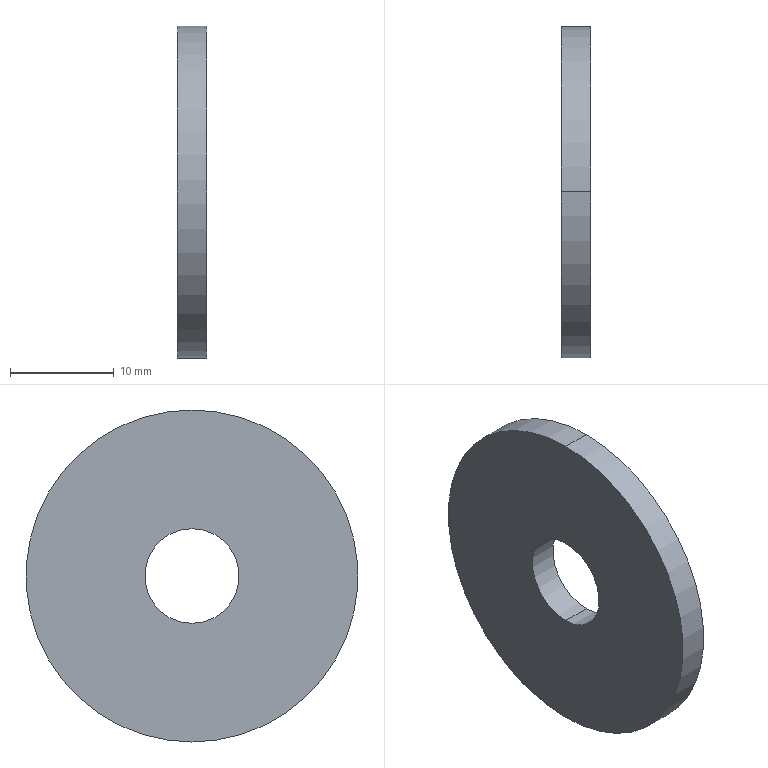Part | STEP file | flat washer wide_am_B18.22M - Plain washer, 8 mm, wide | 1 solid | 6 faces | box 2.8 x 32 x 32 mm | volume 2069 mm3 | cylinder 4 | plane 2 | commonest cylinder face diameters 9.12 x2 32 x2
STEP:
#1=CARTESIAN_POINT('',(0.,0.,0.));
#2=DIRECTION('',(0.,0.,1.));
#3=DIRECTION('',(1.,0.,0.));
#4=AXIS2_PLACEMENT_3D('',#1,#2,#3);
#5=CARTESIAN_POINT('',(0.,0.,16.));
#6=VERTEX_POINT('',#5);
#7=CARTESIAN_POINT('',(0.,0.,-16.));
#8=VERTEX_POINT('',#7);
#9=CARTESIAN_POINT('',(0.,0.,0.));
#10=DIRECTION('',(-1.,0.,0.));
#11=DIRECTION('',(0.,0.,1.));
#12=AXIS2_PLACEMENT_3D('',#9,#10,#11);
#13=CIRCLE('',#12,16.);
#14=CARTESIAN_POINT('',(-34.925,0.,0.));
#15=DIRECTION('',(-1.,0.,0.));
#16=DIRECTION('',(0.,0.,1.));
#17=AXIS2_PLACEMENT_3D('',#14,#15,#16);
#18=CYLINDRICAL_SURFACE('',#17,16.);
#19=CARTESIAN_POINT('',(0.,-34.925));
#20=DIRECTION('',(1.,0.));
#21=VECTOR('',#20,1.);
#22=LINE('',#19,#21);
#23=(GEOMETRIC_REPRESENTATION_CONTEXT(2)PARAMETRIC_REPRESENTATION_CONTEXT()REPRESENTATION_CONTEXT('',''));
#24=DEFINITIONAL_REPRESENTATION('',(#22),#23);
#25=PCURVE('',#18,#24);
#26=CARTESIAN_POINT('',(0.,4.56,0.));
#27=DIRECTION('',(-1.,0.,0.));
#28=DIRECTION('',(0.,0.,1.));
#29=AXIS2_PLACEMENT_3D('',#26,#27,#28);
#30=PLANE('',#29);
#31=CARTESIAN_POINT('',(0.,-4.56));
#32=DIRECTION('',(1.,0.));
#33=AXIS2_PLACEMENT_2D('',#31,#32);
#34=CIRCLE('',#33,16.);
#35=(GEOMETRIC_REPRESENTATION_CONTEXT(2)PARAMETRIC_REPRESENTATION_CONTEXT()REPRESENTATION_CONTEXT('',''));
#36=DEFINITIONAL_REPRESENTATION('',(#34),#35);
#37=PCURVE('',#30,#36);
#38=SURFACE_CURVE('',#13,(#25,#37),.PCURVE_S1.);
#39=EDGE_CURVE('',#6,#8,#38,.T.);
#40=ORIENTED_EDGE('',*,*,#39,.T.);
#41=CARTESIAN_POINT('',(-2.8,0.,-16.));
#42=VERTEX_POINT('',#41);
#43=CARTESIAN_POINT('',(-34.925,0.,-16.));
#44=DIRECTION('',(-1.,0.,0.));
#45=VECTOR('',#44,1.);
#46=LINE('',#43,#45);
#47=CARTESIAN_POINT('',(3.142,0.));
#48=DIRECTION('',(0.,1.));
#49=VECTOR('',#48,1.);
#50=LINE('',#47,#49);
#51=(GEOMETRIC_REPRESENTATION_CONTEXT(2)PARAMETRIC_REPRESENTATION_CONTEXT()REPRESENTATION_CONTEXT('',''));
#52=DEFINITIONAL_REPRESENTATION('',(#50),#51);
#53=PCURVE('',#18,#52);
#54=CARTESIAN_POINT('',(-34.925,0.,0.));
#55=DIRECTION('',(-1.,0.,0.));
#56=DIRECTION('',(0.,0.,1.));
#57=AXIS2_PLACEMENT_3D('',#54,#55,#56);
#58=CYLINDRICAL_SURFACE('',#57,16.);
#59=CARTESIAN_POINT('',(3.142,0.));
#60=DIRECTION('',(0.,1.));
#61=VECTOR('',#60,1.);
#62=LINE('',#59,#61);
#63=(GEOMETRIC_REPRESENTATION_CONTEXT(2)PARAMETRIC_REPRESENTATION_CONTEXT()REPRESENTATION_CONTEXT('',''));
#64=DEFINITIONAL_REPRESENTATION('',(#62),#63);
#65=PCURVE('',#58,#64);
#66=SURFACE_CURVE('',#46,(#53,#65),.PCURVE_S1.);
#67=EDGE_CURVE('',#8,#42,#66,.T.);
#68=ORIENTED_EDGE('',*,*,#67,.T.);
#69=CARTESIAN_POINT('',(-2.8,0.,16.));
#70=VERTEX_POINT('',#69);
#71=CARTESIAN_POINT('',(-2.8,0.,0.));
#72=DIRECTION('',(-1.,0.,0.));
#73=DIRECTION('',(0.,0.,1.));
#74=AXIS2_PLACEMENT_3D('',#71,#72,#73);
#75=CIRCLE('',#74,16.);
#76=CARTESIAN_POINT('',(0.,-32.125));
#77=DIRECTION('',(1.,0.));
#78=VECTOR('',#77,1.);
#79=LINE('',#76,#78);
#80=(GEOMETRIC_REPRESENTATION_CONTEXT(2)PARAMETRIC_REPRESENTATION_CONTEXT()REPRESENTATION_CONTEXT('',''));
#81=DEFINITIONAL_REPRESENTATION('',(#79),#80);
#82=PCURVE('',#18,#81);
#83=CARTESIAN_POINT('',(-2.8,16.,0.));
#84=DIRECTION('',(1.,0.,0.));
#85=DIRECTION('',(0.,0.,-1.));
#86=AXIS2_PLACEMENT_3D('',#83,#84,#85);
#87=PLANE('',#86);
#88=CARTESIAN_POINT('',(-16.,-16.));
#89=CARTESIAN_POINT('',(-16.,11.713));
#90=CARTESIAN_POINT('',(8.,-2.144));
#91=CARTESIAN_POINT('',(32.,-16.));
#92=CARTESIAN_POINT('',(8.,-29.856));
#93=CARTESIAN_POINT('',(-16.,-43.713));
#94=CARTESIAN_POINT('',(-16.,-16.));
#95=(BOUNDED_CURVE()B_SPLINE_CURVE(2,(#88,#89,#90,#91,#92,#93,#94),.UNSPECIFIED.,.T.,.F.)B_SPLINE_CURVE_WITH_KNOTS((1,2,2,2,2,1),(-2.094,0.,2.094,4.189,6.283,8.378),.UNSPECIFIED.)CURVE()GEOMETRIC_REPRESENTATION_ITEM()RATIONAL_B_SPLINE_CURVE((1.,0.5,1.,0.5,1.,0.5,1.))REPRESENTATION_ITEM(''));
#96=(GEOMETRIC_REPRESENTATION_CONTEXT(2)PARAMETRIC_REPRESENTATION_CONTEXT()REPRESENTATION_CONTEXT('',''));
#97=DEFINITIONAL_REPRESENTATION('',(#95),#96);
#98=PCURVE('',#87,#97);
#99=SURFACE_CURVE('',#75,(#82,#98),.PCURVE_S1.);
#100=EDGE_CURVE('',#70,#42,#99,.T.);
#101=ORIENTED_EDGE('',*,*,#100,.F.);
#102=CARTESIAN_POINT('',(-34.925,0.,16.));
#103=DIRECTION('',(-1.,0.,0.));
#104=VECTOR('',#103,1.);
#105=LINE('',#102,#104);
#106=CARTESIAN_POINT('',(0.,0.));
#107=DIRECTION('',(0.,1.));
#108=VECTOR('',#107,1.);
#109=LINE('',#106,#108);
#110=(GEOMETRIC_REPRESENTATION_CONTEXT(2)PARAMETRIC_REPRESENTATION_CONTEXT()REPRESENTATION_CONTEXT('',''));
#111=DEFINITIONAL_REPRESENTATION('',(#109),#110);
#112=PCURVE('',#18,#111);
#113=CARTESIAN_POINT('',(6.283,0.));
#114=DIRECTION('',(0.,1.));
#115=VECTOR('',#114,1.);
#116=LINE('',#113,#115);
#117=(GEOMETRIC_REPRESENTATION_CONTEXT(2)PARAMETRIC_REPRESENTATION_CONTEXT()REPRESENTATION_CONTEXT('',''));
#118=DEFINITIONAL_REPRESENTATION('',(#116),#117);
#119=PCURVE('',#58,#118);
#120=SURFACE_CURVE('',#105,(#112,#119),.PCURVE_S1.);
#121=EDGE_CURVE('',#6,#70,#120,.T.);
#122=ORIENTED_EDGE('',*,*,#121,.F.);
#123=EDGE_LOOP('',(#40,#68,#101,#122));
#124=FACE_BOUND('',#123,.T.);
#125=ADVANCED_FACE('',(#124),#18,.T.);
#126=CARTESIAN_POINT('',(0.,0.,4.56));
#127=VERTEX_POINT('',#126);
#128=CARTESIAN_POINT('',(-2.8,0.,4.56));
#129=VERTEX_POINT('',#128);
#130=CARTESIAN_POINT('',(-34.925,0.,4.56));
#131=DIRECTION('',(-1.,0.,0.));
#132=VECTOR('',#131,1.);
#133=LINE('',#130,#132);
#134=CARTESIAN_POINT('',(-34.925,0.,0.));
#135=DIRECTION('',(-1.,0.,0.));
#136=DIRECTION('',(0.,0.,1.));
#137=AXIS2_PLACEMENT_3D('',#134,#135,#136);
#138=CYLINDRICAL_SURFACE('',#137,4.56);
#139=CARTESIAN_POINT('',(6.283,0.));
#140=DIRECTION('',(0.,1.));
#141=VECTOR('',#140,1.);
#142=LINE('',#139,#141);
#143=(GEOMETRIC_REPRESENTATION_CONTEXT(2)PARAMETRIC_REPRESENTATION_CONTEXT()REPRESENTATION_CONTEXT('',''));
#144=DEFINITIONAL_REPRESENTATION('',(#142),#143);
#145=PCURVE('',#138,#144);
#146=CARTESIAN_POINT('',(-34.925,0.,0.));
#147=DIRECTION('',(-1.,0.,0.));
#148=DIRECTION('',(0.,0.,1.));
#149=AXIS2_PLACEMENT_3D('',#146,#147,#148);
#150=CYLINDRICAL_SURFACE('',#149,4.56);
#151=CARTESIAN_POINT('',(0.,0.));
#152=DIRECTION('',(0.,1.));
#153=VECTOR('',#152,1.);
#154=LINE('',#151,#153);
#155=(GEOMETRIC_REPRESENTATION_CONTEXT(2)PARAMETRIC_REPRESENTATION_CONTEXT()REPRESENTATION_CONTEXT('',''));
#156=DEFINITIONAL_REPRESENTATION('',(#154),#155);
#157=PCURVE('',#150,#156);
#158=SURFACE_CURVE('',#133,(#145,#157),.PCURVE_S1.);
#159=EDGE_CURVE('',#127,#129,#158,.T.);
#160=ORIENTED_EDGE('',*,*,#159,.T.);
#161=CARTESIAN_POINT('',(-2.8,0.,-4.56));
#162=VERTEX_POINT('',#161);
#163=CARTESIAN_POINT('',(-2.8,0.,0.));
#164=DIRECTION('',(-1.,0.,0.));
#165=DIRECTION('',(0.,0.,1.));
#166=AXIS2_PLACEMENT_3D('',#163,#164,#165);
#167=CIRCLE('',#166,4.56);
#168=CARTESIAN_POINT('',(0.,-32.125));
#169=DIRECTION('',(1.,0.));
#170=VECTOR('',#169,1.);
#171=LINE('',#168,#170);
#172=(GEOMETRIC_REPRESENTATION_CONTEXT(2)PARAMETRIC_REPRESENTATION_CONTEXT()REPRESENTATION_CONTEXT('',''));
#173=DEFINITIONAL_REPRESENTATION('',(#171),#172);
#174=PCURVE('',#138,#173);
#175=CARTESIAN_POINT('',(-4.56,-16.));
#176=CARTESIAN_POINT('',(-4.56,-8.102));
#177=CARTESIAN_POINT('',(2.28,-12.051));
#178=CARTESIAN_POINT('',(9.12,-16.));
#179=CARTESIAN_POINT('',(2.28,-19.949));
#180=CARTESIAN_POINT('',(-4.56,-23.898));
#181=CARTESIAN_POINT('',(-4.56,-16.));
#182=(BOUNDED_CURVE()B_SPLINE_CURVE(2,(#175,#176,#177,#178,#179,#180,#181),.UNSPECIFIED.,.T.,.F.)B_SPLINE_CURVE_WITH_KNOTS((1,2,2,2,2,1),(-2.094,0.,2.094,4.189,6.283,8.378),.UNSPECIFIED.)CURVE()GEOMETRIC_REPRESENTATION_ITEM()RATIONAL_B_SPLINE_CURVE((1.,0.5,1.,0.5,1.,0.5,1.))REPRESENTATION_ITEM(''));
#183=(GEOMETRIC_REPRESENTATION_CONTEXT(2)PARAMETRIC_REPRESENTATION_CONTEXT()REPRESENTATION_CONTEXT('',''));
#184=DEFINITIONAL_REPRESENTATION('',(#182),#183);
#185=PCURVE('',#87,#184);
#186=SURFACE_CURVE('',#167,(#174,#185),.PCURVE_S1.);
#187=EDGE_CURVE('',#162,#129,#186,.T.);
#188=ORIENTED_EDGE('',*,*,#187,.F.);
#189=CARTESIAN_POINT('',(0.,0.,-4.56));
#190=VERTEX_POINT('',#189);
#191=CARTESIAN_POINT('',(-34.925,0.,-4.56));
#192=DIRECTION('',(-1.,0.,0.));
#193=VECTOR('',#192,1.);
#194=LINE('',#191,#193);
#195=CARTESIAN_POINT('',(3.142,0.));
#196=DIRECTION('',(0.,1.));
#197=VECTOR('',#196,1.);
#198=LINE('',#195,#197);
#199=(GEOMETRIC_REPRESENTATION_CONTEXT(2)PARAMETRIC_REPRESENTATION_CONTEXT()REPRESENTATION_CONTEXT('',''));
#200=DEFINITIONAL_REPRESENTATION('',(#198),#199);
#201=PCURVE('',#138,#200);
#202=CARTESIAN_POINT('',(3.142,0.));
#203=DIRECTION('',(0.,1.));
#204=VECTOR('',#203,1.);
#205=LINE('',#202,#204);
#206=(GEOMETRIC_REPRESENTATION_CONTEXT(2)PARAMETRIC_REPRESENTATION_CONTEXT()REPRESENTATION_CONTEXT('',''));
#207=DEFINITIONAL_REPRESENTATION('',(#205),#206);
#208=PCURVE('',#150,#207);
#209=SURFACE_CURVE('',#194,(#201,#208),.PCURVE_S1.);
#210=EDGE_CURVE('',#190,#162,#209,.T.);
#211=ORIENTED_EDGE('',*,*,#210,.F.);
#212=CARTESIAN_POINT('',(0.,0.,0.));
#213=DIRECTION('',(-1.,0.,0.));
#214=DIRECTION('',(0.,0.,1.));
#215=AXIS2_PLACEMENT_3D('',#212,#213,#214);
#216=CIRCLE('',#215,4.56);
#217=CARTESIAN_POINT('',(0.,-34.925));
#218=DIRECTION('',(1.,0.));
#219=VECTOR('',#218,1.);
#220=LINE('',#217,#219);
#221=(GEOMETRIC_REPRESENTATION_CONTEXT(2)PARAMETRIC_REPRESENTATION_CONTEXT()REPRESENTATION_CONTEXT('',''));
#222=DEFINITIONAL_REPRESENTATION('',(#220),#221);
#223=PCURVE('',#138,#222);
#224=CARTESIAN_POINT('',(0.,-4.56));
#225=DIRECTION('',(1.,0.));
#226=AXIS2_PLACEMENT_2D('',#224,#225);
#227=CIRCLE('',#226,4.56);
#228=(GEOMETRIC_REPRESENTATION_CONTEXT(2)PARAMETRIC_REPRESENTATION_CONTEXT()REPRESENTATION_CONTEXT('',''));
#229=DEFINITIONAL_REPRESENTATION('',(#227),#228);
#230=PCURVE('',#30,#229);
#231=SURFACE_CURVE('',#216,(#223,#230),.PCURVE_S1.);
#232=EDGE_CURVE('',#190,#127,#231,.T.);
#233=ORIENTED_EDGE('',*,*,#232,.T.);
#234=EDGE_LOOP('',(#160,#188,#211,#233));
#235=FACE_BOUND('',#234,.F.);
#236=ADVANCED_FACE('',(#235),#138,.F.);
#237=CARTESIAN_POINT('',(-2.8,0.,0.));
#238=DIRECTION('',(-1.,0.,0.));
#239=DIRECTION('',(0.,0.,1.));
#240=AXIS2_PLACEMENT_3D('',#237,#238,#239);
#241=CIRCLE('',#240,4.56);
#242=CARTESIAN_POINT('',(0.,-32.125));
#243=DIRECTION('',(1.,0.));
#244=VECTOR('',#243,1.);
#245=LINE('',#242,#244);
#246=(GEOMETRIC_REPRESENTATION_CONTEXT(2)PARAMETRIC_REPRESENTATION_CONTEXT()REPRESENTATION_CONTEXT('',''));
#247=DEFINITIONAL_REPRESENTATION('',(#245),#246);
#248=PCURVE('',#150,#247);
#249=CARTESIAN_POINT('',(-4.56,-16.));
#250=CARTESIAN_POINT('',(-4.56,-8.102));
#251=CARTESIAN_POINT('',(2.28,-12.051));
#252=CARTESIAN_POINT('',(9.12,-16.));
#253=CARTESIAN_POINT('',(2.28,-19.949));
#254=CARTESIAN_POINT('',(-4.56,-23.898));
#255=CARTESIAN_POINT('',(-4.56,-16.));
#256=(BOUNDED_CURVE()B_SPLINE_CURVE(2,(#249,#250,#251,#252,#253,#254,#255),.UNSPECIFIED.,.T.,.F.)B_SPLINE_CURVE_WITH_KNOTS((1,2,2,2,2,1),(-2.094,0.,2.094,4.189,6.283,8.378),.UNSPECIFIED.)CURVE()GEOMETRIC_REPRESENTATION_ITEM()RATIONAL_B_SPLINE_CURVE((1.,0.5,1.,0.5,1.,0.5,1.))REPRESENTATION_ITEM(''));
#257=(GEOMETRIC_REPRESENTATION_CONTEXT(2)PARAMETRIC_REPRESENTATION_CONTEXT()REPRESENTATION_CONTEXT('',''));
#258=DEFINITIONAL_REPRESENTATION('',(#256),#257);
#259=PCURVE('',#87,#258);
#260=SURFACE_CURVE('',#241,(#248,#259),.PCURVE_S1.);
#261=EDGE_CURVE('',#129,#162,#260,.T.);
#262=ORIENTED_EDGE('',*,*,#261,.F.);
#263=ORIENTED_EDGE('',*,*,#159,.F.);
#264=CARTESIAN_POINT('',(0.,0.,0.));
#265=DIRECTION('',(-1.,0.,0.));
#266=DIRECTION('',(0.,0.,1.));
#267=AXIS2_PLACEMENT_3D('',#264,#265,#266);
#268=CIRCLE('',#267,4.56);
#269=CARTESIAN_POINT('',(0.,-34.925));
#270=DIRECTION('',(1.,0.));
#271=VECTOR('',#270,1.);
#272=LINE('',#269,#271);
#273=(GEOMETRIC_REPRESENTATION_CONTEXT(2)PARAMETRIC_REPRESENTATION_CONTEXT()REPRESENTATION_CONTEXT('',''));
#274=DEFINITIONAL_REPRESENTATION('',(#272),#273);
#275=PCURVE('',#150,#274);
#276=CARTESIAN_POINT('',(0.,-4.56));
#277=DIRECTION('',(1.,0.));
#278=AXIS2_PLACEMENT_2D('',#276,#277);
#279=CIRCLE('',#278,4.56);
#280=(GEOMETRIC_REPRESENTATION_CONTEXT(2)PARAMETRIC_REPRESENTATION_CONTEXT()REPRESENTATION_CONTEXT('',''));
#281=DEFINITIONAL_REPRESENTATION('',(#279),#280);
#282=PCURVE('',#30,#281);
#283=SURFACE_CURVE('',#268,(#275,#282),.PCURVE_S1.);
#284=EDGE_CURVE('',#127,#190,#283,.T.);
#285=ORIENTED_EDGE('',*,*,#284,.T.);
#286=ORIENTED_EDGE('',*,*,#210,.T.);
#287=EDGE_LOOP('',(#262,#263,#285,#286));
#288=FACE_BOUND('',#287,.F.);
#289=ADVANCED_FACE('',(#288),#150,.F.);
#290=ORIENTED_EDGE('',*,*,#39,.F.);
#291=CARTESIAN_POINT('',(0.,0.,0.));
#292=DIRECTION('',(-1.,0.,0.));
#293=DIRECTION('',(0.,0.,1.));
#294=AXIS2_PLACEMENT_3D('',#291,#292,#293);
#295=CIRCLE('',#294,16.);
#296=CARTESIAN_POINT('',(0.,-4.56));
#297=DIRECTION('',(1.,0.));
#298=AXIS2_PLACEMENT_2D('',#296,#297);
#299=CIRCLE('',#298,16.);
#300=(GEOMETRIC_REPRESENTATION_CONTEXT(2)PARAMETRIC_REPRESENTATION_CONTEXT()REPRESENTATION_CONTEXT('',''));
#301=DEFINITIONAL_REPRESENTATION('',(#299),#300);
#302=PCURVE('',#30,#301);
#303=CARTESIAN_POINT('',(0.,-34.925));
#304=DIRECTION('',(1.,0.));
#305=VECTOR('',#304,1.);
#306=LINE('',#303,#305);
#307=(GEOMETRIC_REPRESENTATION_CONTEXT(2)PARAMETRIC_REPRESENTATION_CONTEXT()REPRESENTATION_CONTEXT('',''));
#308=DEFINITIONAL_REPRESENTATION('',(#306),#307);
#309=PCURVE('',#58,#308);
#310=SURFACE_CURVE('',#295,(#302,#309),.PCURVE_S1.);
#311=EDGE_CURVE('',#8,#6,#310,.T.);
#312=ORIENTED_EDGE('',*,*,#311,.F.);
#313=EDGE_LOOP('',(#290,#312));
#314=FACE_BOUND('',#313,.T.);
#315=ORIENTED_EDGE('',*,*,#284,.T.);
#316=ORIENTED_EDGE('',*,*,#232,.T.);
#317=EDGE_LOOP('',(#315,#316));
#318=FACE_BOUND('',#317,.T.);
#319=ADVANCED_FACE('',(#314,#318),#30,.F.);
#320=ORIENTED_EDGE('',*,*,#67,.F.);
#321=ORIENTED_EDGE('',*,*,#311,.T.);
#322=ORIENTED_EDGE('',*,*,#121,.T.);
#323=CARTESIAN_POINT('',(-2.8,0.,0.));
#324=DIRECTION('',(-1.,0.,0.));
#325=DIRECTION('',(0.,0.,1.));
#326=AXIS2_PLACEMENT_3D('',#323,#324,#325);
#327=CIRCLE('',#326,16.);
#328=CARTESIAN_POINT('',(0.,-32.125));
#329=DIRECTION('',(1.,0.));
#330=VECTOR('',#329,1.);
#331=LINE('',#328,#330);
#332=(GEOMETRIC_REPRESENTATION_CONTEXT(2)PARAMETRIC_REPRESENTATION_CONTEXT()REPRESENTATION_CONTEXT('',''));
#333=DEFINITIONAL_REPRESENTATION('',(#331),#332);
#334=PCURVE('',#58,#333);
#335=CARTESIAN_POINT('',(-16.,-16.));
#336=CARTESIAN_POINT('',(-16.,11.713));
#337=CARTESIAN_POINT('',(8.,-2.144));
#338=CARTESIAN_POINT('',(32.,-16.));
#339=CARTESIAN_POINT('',(8.,-29.856));
#340=CARTESIAN_POINT('',(-16.,-43.713));
#341=CARTESIAN_POINT('',(-16.,-16.));
#342=(BOUNDED_CURVE()B_SPLINE_CURVE(2,(#335,#336,#337,#338,#339,#340,#341),.UNSPECIFIED.,.T.,.F.)B_SPLINE_CURVE_WITH_KNOTS((1,2,2,2,2,1),(-2.094,0.,2.094,4.189,6.283,8.378),.UNSPECIFIED.)CURVE()GEOMETRIC_REPRESENTATION_ITEM()RATIONAL_B_SPLINE_CURVE((1.,0.5,1.,0.5,1.,0.5,1.))REPRESENTATION_ITEM(''));
#343=(GEOMETRIC_REPRESENTATION_CONTEXT(2)PARAMETRIC_REPRESENTATION_CONTEXT()REPRESENTATION_CONTEXT('',''));
#344=DEFINITIONAL_REPRESENTATION('',(#342),#343);
#345=PCURVE('',#87,#344);
#346=SURFACE_CURVE('',#327,(#334,#345),.PCURVE_S1.);
#347=EDGE_CURVE('',#42,#70,#346,.T.);
#348=ORIENTED_EDGE('',*,*,#347,.F.);
#349=EDGE_LOOP('',(#320,#321,#322,#348));
#350=FACE_BOUND('',#349,.T.);
#351=ADVANCED_FACE('',(#350),#58,.T.);
#352=ORIENTED_EDGE('',*,*,#261,.F.);
#353=ORIENTED_EDGE('',*,*,#187,.F.);
#354=EDGE_LOOP('',(#352,#353));
#355=FACE_BOUND('',#354,.T.);
#356=ORIENTED_EDGE('',*,*,#100,.T.);
#357=ORIENTED_EDGE('',*,*,#347,.T.);
#358=EDGE_LOOP('',(#356,#357));
#359=FACE_BOUND('',#358,.T.);
#360=ADVANCED_FACE('',(#355,#359),#87,.F.);
#361=CLOSED_SHELL('',(#125,#236,#289,#319,#351,#360));
#362=MANIFOLD_SOLID_BREP('',#361);
#363=(LENGTH_UNIT()NAMED_UNIT(*)SI_UNIT(.MILLI.,.METRE.));
#364=UNCERTAINTY_MEASURE_WITH_UNIT(LENGTH_MEASURE(0.0000001),#363,'','');
#365=(NAMED_UNIT(*)PLANE_ANGLE_UNIT()SI_UNIT($,.RADIAN.));
#366=(NAMED_UNIT(*)SI_UNIT($,.STERADIAN.)SOLID_ANGLE_UNIT());
#367=(GEOMETRIC_REPRESENTATION_CONTEXT(3)GLOBAL_UNCERTAINTY_ASSIGNED_CONTEXT((#364))GLOBAL_UNIT_ASSIGNED_CONTEXT((#363,#365,#366))REPRESENTATION_CONTEXT('',''));
#368=ADVANCED_BREP_SHAPE_REPRESENTATION('',(#4,#362),#367);